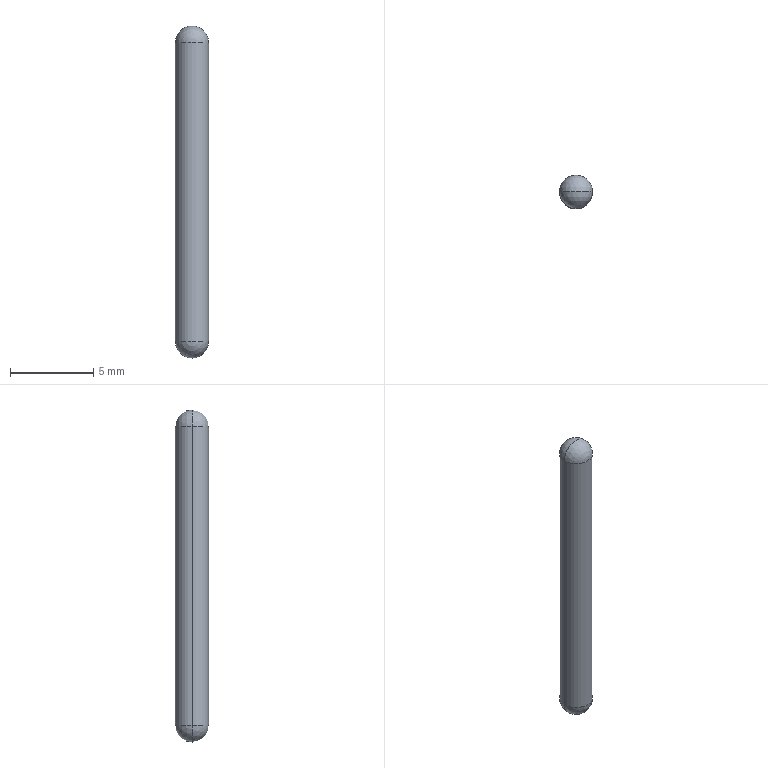Part | SolidWorks | features Extrusion 1, Fillet 1 | 1 solid | 6 faces | box 2 x 2 x 20 mm | volume 60.737 mm3 | sphere 4 | cylinder 2 | commonest cylinder face diameters 2 x2
STEP:
#1=CARTESIAN_POINT('',(-92.3,42.,-6.));
#2=VERTEX_POINT('',#1);
#3=CARTESIAN_POINT('',(-90.3,42.,-6.));
#4=VERTEX_POINT('',#3);
#5=CARTESIAN_POINT('',(-91.3,42.,-6.));
#6=DIRECTION('',(0.,0.,-1.));
#7=DIRECTION('',(1.,0.,0.));
#8=AXIS2_PLACEMENT_3D('',#5,#6,#7);
#9=CIRCLE('',#8,1.);
#10=EDGE_CURVE('',#2,#4,#9,.T.);
#11=ORIENTED_EDGE('',*,*,#10,.F.);
#12=CARTESIAN_POINT('',(-91.3,42.,-5.));
#13=VERTEX_POINT('',#12);
#14=CARTESIAN_POINT('',(-91.3,42.,-6.));
#15=DIRECTION('',(0.,1.,0.));
#16=DIRECTION('',(-1.,0.,0.));
#17=AXIS2_PLACEMENT_3D('',#14,#15,#16);
#18=CIRCLE('',#17,1.);
#19=EDGE_CURVE('',#2,#13,#18,.T.);
#20=ORIENTED_EDGE('',*,*,#19,.T.);
#21=CARTESIAN_POINT('',(-91.3,42.,-6.));
#22=DIRECTION('',(0.,-1.,0.));
#23=DIRECTION('',(0.,0.,-1.));
#24=AXIS2_PLACEMENT_3D('',#21,#22,#23);
#25=CIRCLE('',#24,1.);
#26=EDGE_CURVE('',#4,#13,#25,.T.);
#27=ORIENTED_EDGE('',*,*,#26,.F.);
#28=EDGE_LOOP('',(#11,#20,#27));
#29=FACE_OUTER_BOUND('',#28,.T.);
#30=CARTESIAN_POINT('',(-91.3,42.,-6.));
#31=DIRECTION('',(0.,1.,0.));
#32=DIRECTION('',(1.,0.,0.));
#33=AXIS2_PLACEMENT_3D('',#30,#31,#32);
#34=SPHERICAL_SURFACE('',#33,1.);
#35=ADVANCED_FACE('',(#29),#34,.T.);
#36=CARTESIAN_POINT('',(-91.3,42.,-25.));
#37=VERTEX_POINT('',#36);
#38=CARTESIAN_POINT('',(-90.3,42.,-24.));
#39=VERTEX_POINT('',#38);
#40=CARTESIAN_POINT('',(-91.3,42.,-24.));
#41=DIRECTION('',(0.,-1.,0.));
#42=DIRECTION('',(0.,0.,-1.));
#43=AXIS2_PLACEMENT_3D('',#40,#41,#42);
#44=CIRCLE('',#43,1.);
#45=EDGE_CURVE('',#37,#39,#44,.T.);
#46=ORIENTED_EDGE('',*,*,#45,.F.);
#47=CARTESIAN_POINT('',(-92.3,42.,-24.));
#48=VERTEX_POINT('',#47);
#49=CARTESIAN_POINT('',(-91.3,42.,-24.));
#50=DIRECTION('',(0.,1.,0.));
#51=DIRECTION('',(-1.,0.,0.));
#52=AXIS2_PLACEMENT_3D('',#49,#50,#51);
#53=CIRCLE('',#52,1.);
#54=EDGE_CURVE('',#37,#48,#53,.T.);
#55=ORIENTED_EDGE('',*,*,#54,.T.);
#56=CARTESIAN_POINT('',(-91.3,42.,-24.));
#57=DIRECTION('',(0.,0.,1.));
#58=DIRECTION('',(1.,0.,0.));
#59=AXIS2_PLACEMENT_3D('',#56,#57,#58);
#60=CIRCLE('',#59,1.);
#61=EDGE_CURVE('',#39,#48,#60,.T.);
#62=ORIENTED_EDGE('',*,*,#61,.F.);
#63=EDGE_LOOP('',(#46,#55,#62));
#64=FACE_OUTER_BOUND('',#63,.T.);
#65=CARTESIAN_POINT('',(-91.3,42.,-24.));
#66=DIRECTION('',(0.,1.,0.));
#67=DIRECTION('',(1.,0.,0.));
#68=AXIS2_PLACEMENT_3D('',#65,#66,#67);
#69=SPHERICAL_SURFACE('',#68,1.);
#70=ADVANCED_FACE('',(#64),#69,.T.);
#71=ORIENTED_EDGE('',*,*,#61,.T.);
#72=CARTESIAN_POINT('',(-92.3,42.,-25.));
#73=DIRECTION('',(0.,0.,1.));
#74=VECTOR('',#73,1000.);
#75=LINE('',#72,#74);
#76=EDGE_CURVE('',#48,#2,#75,.T.);
#77=ORIENTED_EDGE('',*,*,#76,.T.);
#78=ORIENTED_EDGE('',*,*,#10,.T.);
#79=CARTESIAN_POINT('',(-90.3,42.,-25.));
#80=DIRECTION('',(0.,0.,1.));
#81=VECTOR('',#80,1000.);
#82=LINE('',#79,#81);
#83=EDGE_CURVE('',#39,#4,#82,.T.);
#84=ORIENTED_EDGE('',*,*,#83,.F.);
#85=EDGE_LOOP('',(#71,#77,#78,#84));
#86=FACE_OUTER_BOUND('',#85,.T.);
#87=CARTESIAN_POINT('',(-91.3,42.,-25.));
#88=DIRECTION('',(0.,0.,1.));
#89=DIRECTION('',(1.,0.,0.));
#90=AXIS2_PLACEMENT_3D('',#87,#88,#89);
#91=CYLINDRICAL_SURFACE('',#90,1.);
#92=ADVANCED_FACE('',(#86),#91,.T.);
#93=ORIENTED_EDGE('',*,*,#76,.F.);
#94=CARTESIAN_POINT('',(-91.3,42.,-24.));
#95=DIRECTION('',(0.,0.,1.));
#96=DIRECTION('',(1.,0.,0.));
#97=AXIS2_PLACEMENT_3D('',#94,#95,#96);
#98=CIRCLE('',#97,1.);
#99=EDGE_CURVE('',#48,#39,#98,.T.);
#100=ORIENTED_EDGE('',*,*,#99,.T.);
#101=ORIENTED_EDGE('',*,*,#83,.T.);
#102=CARTESIAN_POINT('',(-91.3,42.,-6.));
#103=DIRECTION('',(0.,0.,-1.));
#104=DIRECTION('',(1.,0.,0.));
#105=AXIS2_PLACEMENT_3D('',#102,#103,#104);
#106=CIRCLE('',#105,1.);
#107=EDGE_CURVE('',#4,#2,#106,.T.);
#108=ORIENTED_EDGE('',*,*,#107,.T.);
#109=EDGE_LOOP('',(#93,#100,#101,#108));
#110=FACE_OUTER_BOUND('',#109,.T.);
#111=CARTESIAN_POINT('',(-91.3,42.,-25.));
#112=DIRECTION('',(0.,0.,1.));
#113=DIRECTION('',(1.,0.,0.));
#114=AXIS2_PLACEMENT_3D('',#111,#112,#113);
#115=CYLINDRICAL_SURFACE('',#114,1.);
#116=ADVANCED_FACE('',(#110),#115,.T.);
#117=ORIENTED_EDGE('',*,*,#54,.F.);
#118=ORIENTED_EDGE('',*,*,#45,.T.);
#119=ORIENTED_EDGE('',*,*,#99,.F.);
#120=EDGE_LOOP('',(#117,#118,#119));
#121=FACE_OUTER_BOUND('',#120,.T.);
#122=CARTESIAN_POINT('',(-91.3,42.,-24.));
#123=DIRECTION('',(0.,1.,0.));
#124=DIRECTION('',(1.,0.,0.));
#125=AXIS2_PLACEMENT_3D('',#122,#123,#124);
#126=SPHERICAL_SURFACE('',#125,1.);
#127=ADVANCED_FACE('',(#121),#126,.T.);
#128=ORIENTED_EDGE('',*,*,#19,.F.);
#129=ORIENTED_EDGE('',*,*,#107,.F.);
#130=ORIENTED_EDGE('',*,*,#26,.T.);
#131=EDGE_LOOP('',(#128,#129,#130));
#132=FACE_OUTER_BOUND('',#131,.T.);
#133=CARTESIAN_POINT('',(-91.3,42.,-6.));
#134=DIRECTION('',(0.,1.,0.));
#135=DIRECTION('',(1.,0.,0.));
#136=AXIS2_PLACEMENT_3D('',#133,#134,#135);
#137=SPHERICAL_SURFACE('',#136,1.);
#138=ADVANCED_FACE('',(#132),#137,.T.);
#139=CLOSED_SHELL('',(#35,#70,#92,#116,#127,#138));
#140=MANIFOLD_SOLID_BREP('',#139);
#141=CARTESIAN_POINT('',(0.,0.,0.));
#142=DIRECTION('',(0.,0.,1.));
#143=DIRECTION('',(1.,0.,0.));
#144=AXIS2_PLACEMENT_3D('',#141,#142,#143);
#145=(LENGTH_UNIT()NAMED_UNIT(*)SI_UNIT(.MILLI.,.METRE.));
#146=UNCERTAINTY_MEASURE_WITH_UNIT(LENGTH_MEASURE(0.00001),#145,'','');
#147=(NAMED_UNIT(*)PLANE_ANGLE_UNIT()SI_UNIT($,.RADIAN.));
#148=(NAMED_UNIT(*)SI_UNIT($,.STERADIAN.)SOLID_ANGLE_UNIT());
#149=(GEOMETRIC_REPRESENTATION_CONTEXT(3)GLOBAL_UNCERTAINTY_ASSIGNED_CONTEXT((#146))GLOBAL_UNIT_ASSIGNED_CONTEXT((#145,#147,#148))REPRESENTATION_CONTEXT('',''));
#150=ADVANCED_BREP_SHAPE_REPRESENTATION('',(#140,#144),#149);